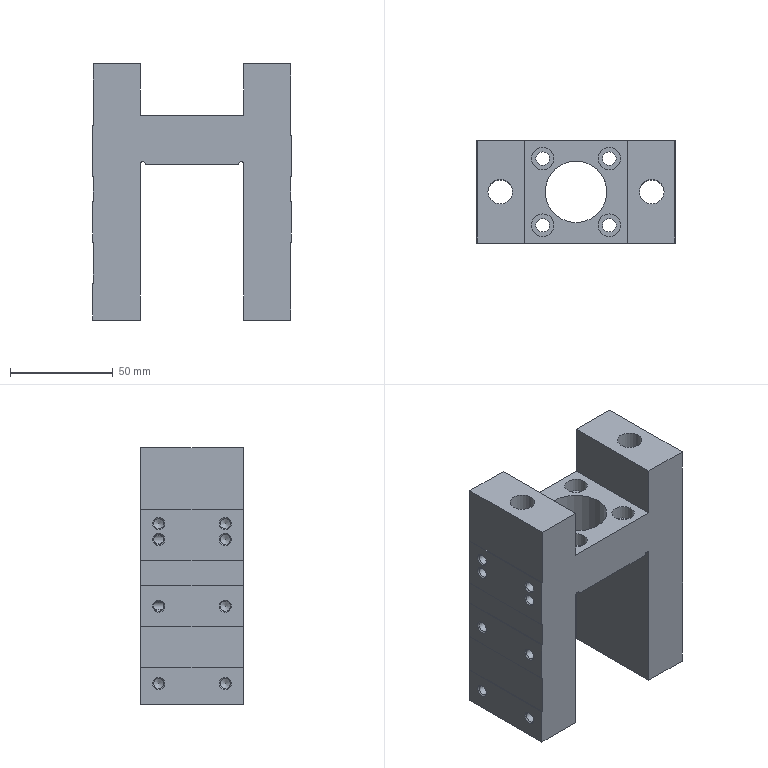Part | STEP file | 150290 FENG-32-KF---(GK) | 1 solid | 101 faces | box 97 x 50 x 125 mm | volume 293495 mm3 | plane 36 | cone 36 | cylinder 29 | commonest cylinder face diameters 4.917 x16 6.6 x4 11 x4 2.5 x2 12 x2 30 x1